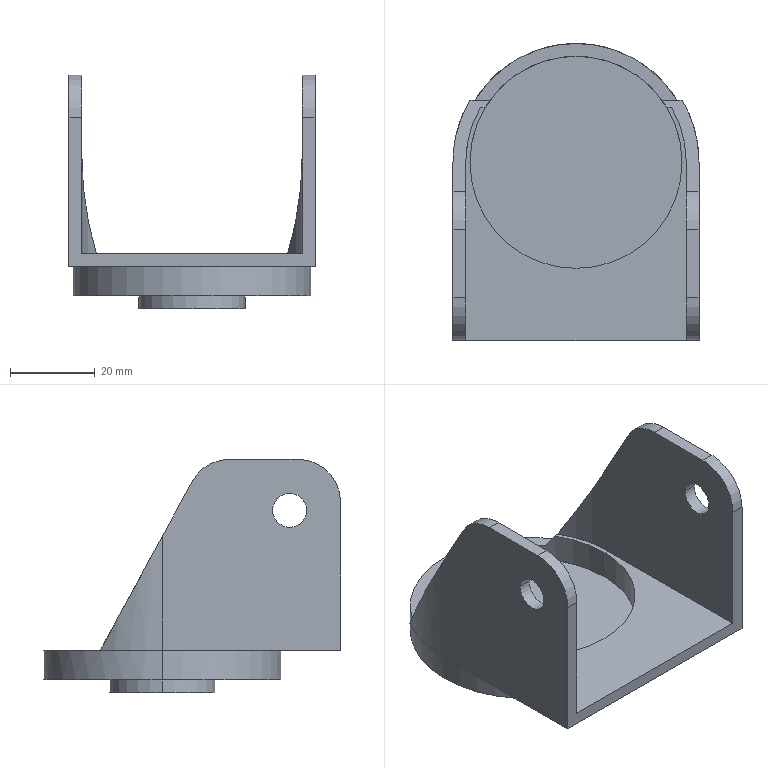Part | SolidWorks | features ICE 7, Extrusion 1, Fillet 1 | 1 solid | 33 faces | box 58 x 70 x 55 mm | volume 26099 mm3 | cylinder 18 | plane 15 | commonest cylinder face diameters 8 x4 20 x4 25 x2 50 x2 52 x2 56 x2
STEP:
#1=CARTESIAN_POINT('',(26.,-26.,43.));
#2=VERTEX_POINT('',#1);
#3=CARTESIAN_POINT('',(26.,-34.,43.));
#4=VERTEX_POINT('',#3);
#5=CARTESIAN_POINT('',(26.,-30.,43.));
#6=DIRECTION('',(-1.,0.,0.));
#7=DIRECTION('',(0.,-1.,0.));
#8=AXIS2_PLACEMENT_3D('',#5,#6,#7);
#9=CIRCLE('',#8,4.);
#10=EDGE_CURVE('',#2,#4,#9,.T.);
#11=ORIENTED_EDGE('',*,*,#10,.T.);
#12=CARTESIAN_POINT('',(29.,-34.,43.));
#13=VERTEX_POINT('',#12);
#14=CARTESIAN_POINT('',(-29.,-34.,43.));
#15=DIRECTION('',(1.,0.,0.));
#16=VECTOR('',#15,1000.);
#17=LINE('',#14,#16);
#18=EDGE_CURVE('',#4,#13,#17,.T.);
#19=ORIENTED_EDGE('',*,*,#18,.T.);
#20=CARTESIAN_POINT('',(29.,-26.,43.));
#21=VERTEX_POINT('',#20);
#22=CARTESIAN_POINT('',(29.,-30.,43.));
#23=DIRECTION('',(1.,0.,0.));
#24=DIRECTION('',(0.,1.,0.));
#25=AXIS2_PLACEMENT_3D('',#22,#23,#24);
#26=CIRCLE('',#25,4.);
#27=EDGE_CURVE('',#13,#21,#26,.T.);
#28=ORIENTED_EDGE('',*,*,#27,.T.);
#29=CARTESIAN_POINT('',(-29.,-26.,43.));
#30=DIRECTION('',(1.,0.,0.));
#31=VECTOR('',#30,1000.);
#32=LINE('',#29,#31);
#33=EDGE_CURVE('',#2,#21,#32,.T.);
#34=ORIENTED_EDGE('',*,*,#33,.F.);
#35=EDGE_LOOP('',(#11,#19,#28,#34));
#36=FACE_OUTER_BOUND('',#35,.T.);
#37=CARTESIAN_POINT('',(-29.,-30.,43.));
#38=DIRECTION('',(1.,0.,0.));
#39=DIRECTION('',(0.,1.,0.));
#40=AXIS2_PLACEMENT_3D('',#37,#38,#39);
#41=CYLINDRICAL_SURFACE('',#40,4.);
#42=ADVANCED_FACE('',(#36),#41,.F.);
#43=CARTESIAN_POINT('',(-29.,-34.,43.));
#44=VERTEX_POINT('',#43);
#45=CARTESIAN_POINT('',(-29.,-26.,43.));
#46=VERTEX_POINT('',#45);
#47=CARTESIAN_POINT('',(-29.,-30.,43.));
#48=DIRECTION('',(1.,0.,0.));
#49=DIRECTION('',(0.,1.,0.));
#50=AXIS2_PLACEMENT_3D('',#47,#48,#49);
#51=CIRCLE('',#50,4.);
#52=EDGE_CURVE('',#44,#46,#51,.T.);
#53=ORIENTED_EDGE('',*,*,#52,.F.);
#54=CARTESIAN_POINT('',(-26.,-34.,43.));
#55=VERTEX_POINT('',#54);
#56=CARTESIAN_POINT('',(-29.,-34.,43.));
#57=DIRECTION('',(1.,0.,0.));
#58=VECTOR('',#57,1000.);
#59=LINE('',#56,#58);
#60=EDGE_CURVE('',#44,#55,#59,.T.);
#61=ORIENTED_EDGE('',*,*,#60,.T.);
#62=CARTESIAN_POINT('',(-26.,-26.,43.));
#63=VERTEX_POINT('',#62);
#64=CARTESIAN_POINT('',(-26.,-30.,43.));
#65=DIRECTION('',(1.,0.,0.));
#66=DIRECTION('',(0.,0.,-1.));
#67=AXIS2_PLACEMENT_3D('',#64,#65,#66);
#68=CIRCLE('',#67,4.);
#69=EDGE_CURVE('',#55,#63,#68,.T.);
#70=ORIENTED_EDGE('',*,*,#69,.T.);
#71=CARTESIAN_POINT('',(-29.,-26.,43.));
#72=DIRECTION('',(1.,0.,0.));
#73=VECTOR('',#72,1000.);
#74=LINE('',#71,#73);
#75=EDGE_CURVE('',#46,#63,#74,.T.);
#76=ORIENTED_EDGE('',*,*,#75,.F.);
#77=EDGE_LOOP('',(#53,#61,#70,#76));
#78=FACE_OUTER_BOUND('',#77,.T.);
#79=CARTESIAN_POINT('',(-29.,-30.,43.));
#80=DIRECTION('',(1.,0.,0.));
#81=DIRECTION('',(0.,1.,0.));
#82=AXIS2_PLACEMENT_3D('',#79,#80,#81);
#83=CYLINDRICAL_SURFACE('',#82,4.);
#84=ADVANCED_FACE('',(#78),#83,.F.);
#85=CARTESIAN_POINT('',(-25.,0.,6.));
#86=VERTEX_POINT('',#85);
#87=CARTESIAN_POINT('',(25.,0.,6.));
#88=VERTEX_POINT('',#87);
#89=CARTESIAN_POINT('',(0.,0.,6.));
#90=DIRECTION('',(0.,0.,1.));
#91=DIRECTION('',(1.,0.,0.));
#92=AXIS2_PLACEMENT_3D('',#89,#90,#91);
#93=CIRCLE('',#92,25.);
#94=EDGE_CURVE('',#86,#88,#93,.T.);
#95=ORIENTED_EDGE('',*,*,#94,.F.);
#96=CARTESIAN_POINT('',(-25.,0.,13.));
#97=VERTEX_POINT('',#96);
#98=CARTESIAN_POINT('',(-25.,0.,6.));
#99=DIRECTION('',(0.,0.,1.));
#100=VECTOR('',#99,1000.);
#101=LINE('',#98,#100);
#102=EDGE_CURVE('',#86,#97,#101,.T.);
#103=ORIENTED_EDGE('',*,*,#102,.T.);
#104=CARTESIAN_POINT('',(25.,0.,13.));
#105=VERTEX_POINT('',#104);
#106=CARTESIAN_POINT('',(0.,0.,13.));
#107=DIRECTION('',(0.,0.,1.));
#108=DIRECTION('',(1.,0.,0.));
#109=AXIS2_PLACEMENT_3D('',#106,#107,#108);
#110=CIRCLE('',#109,25.);
#111=EDGE_CURVE('',#97,#105,#110,.T.);
#112=ORIENTED_EDGE('',*,*,#111,.T.);
#113=CARTESIAN_POINT('',(25.,0.,6.));
#114=DIRECTION('',(0.,0.,1.));
#115=VECTOR('',#114,1000.);
#116=LINE('',#113,#115);
#117=EDGE_CURVE('',#88,#105,#116,.T.);
#118=ORIENTED_EDGE('',*,*,#117,.F.);
#119=EDGE_LOOP('',(#95,#103,#112,#118));
#120=FACE_OUTER_BOUND('',#119,.T.);
#121=CARTESIAN_POINT('',(0.,0.,6.));
#122=DIRECTION('',(0.,0.,1.));
#123=DIRECTION('',(1.,0.,0.));
#124=AXIS2_PLACEMENT_3D('',#121,#122,#123);
#125=CYLINDRICAL_SURFACE('',#124,25.);
#126=ADVANCED_FACE('',(#120),#125,.F.);
#127=CARTESIAN_POINT('',(12.5,0.,3.));
#128=VERTEX_POINT('',#127);
#129=CARTESIAN_POINT('',(-12.5,0.,3.));
#130=VERTEX_POINT('',#129);
#131=CARTESIAN_POINT('',(0.,0.,3.));
#132=DIRECTION('',(0.,0.,1.));
#133=DIRECTION('',(1.,0.,0.));
#134=AXIS2_PLACEMENT_3D('',#131,#132,#133);
#135=CIRCLE('',#134,12.5);
#136=EDGE_CURVE('',#128,#130,#135,.T.);
#137=ORIENTED_EDGE('',*,*,#136,.F.);
#138=CARTESIAN_POINT('',(12.5,0.,0.));
#139=VERTEX_POINT('',#138);
#140=CARTESIAN_POINT('',(12.5,0.,3.));
#141=DIRECTION('',(0.,0.,-1.));
#142=VECTOR('',#141,1000.);
#143=LINE('',#140,#142);
#144=EDGE_CURVE('',#128,#139,#143,.T.);
#145=ORIENTED_EDGE('',*,*,#144,.T.);
#146=CARTESIAN_POINT('',(-12.5,0.,0.));
#147=VERTEX_POINT('',#146);
#148=CARTESIAN_POINT('',(0.,0.,0.));
#149=DIRECTION('',(0.,0.,1.));
#150=DIRECTION('',(1.,0.,0.));
#151=AXIS2_PLACEMENT_3D('',#148,#149,#150);
#152=CIRCLE('',#151,12.5);
#153=EDGE_CURVE('',#139,#147,#152,.T.);
#154=ORIENTED_EDGE('',*,*,#153,.T.);
#155=CARTESIAN_POINT('',(-12.5,0.,3.));
#156=DIRECTION('',(0.,0.,-1.));
#157=VECTOR('',#156,1000.);
#158=LINE('',#155,#157);
#159=EDGE_CURVE('',#130,#147,#158,.T.);
#160=ORIENTED_EDGE('',*,*,#159,.F.);
#161=EDGE_LOOP('',(#137,#145,#154,#160));
#162=FACE_OUTER_BOUND('',#161,.T.);
#163=CARTESIAN_POINT('',(0.,0.,3.));
#164=DIRECTION('',(0.,0.,-1.));
#165=DIRECTION('',(-1.,0.,0.));
#166=AXIS2_PLACEMENT_3D('',#163,#164,#165);
#167=CYLINDRICAL_SURFACE('',#166,12.5);
#168=ADVANCED_FACE('',(#162),#167,.T.);
#169=CARTESIAN_POINT('',(28.,0.,10.));
#170=VERTEX_POINT('',#169);
#171=CARTESIAN_POINT('',(23.886,14.61,10.));
#172=VERTEX_POINT('',#171);
#173=CARTESIAN_POINT('',(0.,0.,10.));
#174=DIRECTION('',(0.,0.,1.));
#175=DIRECTION('',(1.,0.,0.));
#176=AXIS2_PLACEMENT_3D('',#173,#174,#175);
#177=CIRCLE('',#176,28.);
#178=EDGE_CURVE('',#170,#172,#177,.T.);
#179=ORIENTED_EDGE('',*,*,#178,.F.);
#180=CARTESIAN_POINT('',(28.,0.,3.));
#181=VERTEX_POINT('',#180);
#182=CARTESIAN_POINT('',(28.,0.,13.));
#183=DIRECTION('',(0.,0.,-1.));
#184=VECTOR('',#183,1000.);
#185=LINE('',#182,#184);
#186=EDGE_CURVE('',#170,#181,#185,.T.);
#187=ORIENTED_EDGE('',*,*,#186,.T.);
#188=CARTESIAN_POINT('',(-28.,0.,3.));
#189=VERTEX_POINT('',#188);
#190=CARTESIAN_POINT('',(0.,0.,3.));
#191=DIRECTION('',(0.,0.,1.));
#192=DIRECTION('',(1.,0.,0.));
#193=AXIS2_PLACEMENT_3D('',#190,#191,#192);
#194=CIRCLE('',#193,28.);
#195=EDGE_CURVE('',#181,#189,#194,.T.);
#196=ORIENTED_EDGE('',*,*,#195,.T.);
#197=CARTESIAN_POINT('',(-28.,0.,10.));
#198=VERTEX_POINT('',#197);
#199=CARTESIAN_POINT('',(-28.,0.,13.));
#200=DIRECTION('',(0.,0.,-1.));
#201=VECTOR('',#200,1000.);
#202=LINE('',#199,#201);
#203=EDGE_CURVE('',#198,#189,#202,.T.);
#204=ORIENTED_EDGE('',*,*,#203,.F.);
#205=CARTESIAN_POINT('',(-23.886,14.61,10.));
#206=VERTEX_POINT('',#205);
#207=CARTESIAN_POINT('',(0.,0.,10.));
#208=DIRECTION('',(0.,0.,1.));
#209=DIRECTION('',(1.,0.,0.));
#210=AXIS2_PLACEMENT_3D('',#207,#208,#209);
#211=CIRCLE('',#210,28.);
#212=EDGE_CURVE('',#206,#198,#211,.T.);
#213=ORIENTED_EDGE('',*,*,#212,.F.);
#214=CARTESIAN_POINT('',(0.,0.,10.));
#215=DIRECTION('',(0.,0.,1.));
#216=DIRECTION('',(1.,0.,0.));
#217=AXIS2_PLACEMENT_3D('',#214,#215,#216);
#218=CIRCLE('',#217,28.);
#219=EDGE_CURVE('',#172,#206,#218,.T.);
#220=ORIENTED_EDGE('',*,*,#219,.F.);
#221=EDGE_LOOP('',(#179,#187,#196,#204,#213,#220));
#222=FACE_OUTER_BOUND('',#221,.T.);
#223=CARTESIAN_POINT('',(0.,0.,13.));
#224=DIRECTION('',(0.,0.,-1.));
#225=DIRECTION('',(-1.,0.,0.));
#226=AXIS2_PLACEMENT_3D('',#223,#224,#225);
#227=CYLINDRICAL_SURFACE('',#226,28.);
#228=ADVANCED_FACE('',(#222),#227,.T.);
#229=CARTESIAN_POINT('',(29.,0.,36.854));
#230=VERTEX_POINT('',#229);
#231=CARTESIAN_POINT('',(25.051,14.61,10.));
#232=VERTEX_POINT('',#231);
#233=CARTESIAN_POINT('',(29.,0.,36.854));
#234=CARTESIAN_POINT('',(29.,5.164,27.362));
#235=CARTESIAN_POINT('',(27.653,10.149,18.199));
#236=CARTESIAN_POINT('',(25.051,14.61,10.));
#237=(BOUNDED_CURVE()B_SPLINE_CURVE(3,(#233,#234,#235,#236),.UNSPECIFIED.,.F.,.F.)B_SPLINE_CURVE_WITH_KNOTS((4,4),(1.571,2.099),.UNSPECIFIED.)CURVE()GEOMETRIC_REPRESENTATION_ITEM()RATIONAL_B_SPLINE_CURVE((1.,0.9769,0.9769,1.))REPRESENTATION_ITEM(''));
#238=EDGE_CURVE('',#230,#232,#237,.T.);
#239=ORIENTED_EDGE('',*,*,#238,.F.);
#240=CARTESIAN_POINT('',(29.,0.,10.));
#241=VERTEX_POINT('',#240);
#242=CARTESIAN_POINT('',(29.,0.,10.));
#243=DIRECTION('',(0.,0.,1.));
#244=VECTOR('',#243,1000.);
#245=LINE('',#242,#244);
#246=EDGE_CURVE('',#241,#230,#245,.T.);
#247=ORIENTED_EDGE('',*,*,#246,.F.);
#248=CARTESIAN_POINT('',(0.,0.,10.));
#249=DIRECTION('',(0.,0.,1.));
#250=DIRECTION('',(1.,0.,0.));
#251=AXIS2_PLACEMENT_3D('',#248,#249,#250);
#252=CIRCLE('',#251,29.);
#253=EDGE_CURVE('',#241,#232,#252,.T.);
#254=ORIENTED_EDGE('',*,*,#253,.T.);
#255=EDGE_LOOP('',(#239,#247,#254));
#256=FACE_OUTER_BOUND('',#255,.T.);
#257=CARTESIAN_POINT('',(0.,0.,10.));
#258=DIRECTION('',(0.,0.,1.));
#259=DIRECTION('',(1.,0.,0.));
#260=AXIS2_PLACEMENT_3D('',#257,#258,#259);
#261=CYLINDRICAL_SURFACE('',#260,29.);
#262=ADVANCED_FACE('',(#256),#261,.T.);
#263=CARTESIAN_POINT('',(22.53,12.978,13.));
#264=VERTEX_POINT('',#263);
#265=CARTESIAN_POINT('',(26.,0.,36.854));
#266=VERTEX_POINT('',#265);
#267=CARTESIAN_POINT('',(22.53,12.978,13.));
#268=CARTESIAN_POINT('',(24.816,9.008,20.297));
#269=CARTESIAN_POINT('',(26.,4.582,28.432));
#270=CARTESIAN_POINT('',(26.,0.,36.854));
#271=(BOUNDED_CURVE()B_SPLINE_CURVE(3,(#267,#268,#269,#270),.UNSPECIFIED.,.F.,.F.)B_SPLINE_CURVE_WITH_KNOTS((4,4),(1.048,1.571),.UNSPECIFIED.)CURVE()GEOMETRIC_REPRESENTATION_ITEM()RATIONAL_B_SPLINE_CURVE((1.,0.9774,0.9774,1.))REPRESENTATION_ITEM(''));
#272=EDGE_CURVE('',#264,#266,#271,.T.);
#273=ORIENTED_EDGE('',*,*,#272,.F.);
#274=CARTESIAN_POINT('',(26.,0.,13.));
#275=VERTEX_POINT('',#274);
#276=CARTESIAN_POINT('',(0.,0.,13.));
#277=DIRECTION('',(0.,0.,1.));
#278=DIRECTION('',(1.,0.,0.));
#279=AXIS2_PLACEMENT_3D('',#276,#277,#278);
#280=CIRCLE('',#279,26.);
#281=EDGE_CURVE('',#275,#264,#280,.T.);
#282=ORIENTED_EDGE('',*,*,#281,.F.);
#283=CARTESIAN_POINT('',(26.,0.,55.));
#284=DIRECTION('',(0.,0.,-1.));
#285=VECTOR('',#284,1000.);
#286=LINE('',#283,#285);
#287=EDGE_CURVE('',#266,#275,#286,.T.);
#288=ORIENTED_EDGE('',*,*,#287,.F.);
#289=EDGE_LOOP('',(#273,#282,#288));
#290=FACE_OUTER_BOUND('',#289,.T.);
#291=CARTESIAN_POINT('',(0.,0.,55.));
#292=DIRECTION('',(0.,0.,-1.));
#293=DIRECTION('',(-1.,0.,0.));
#294=AXIS2_PLACEMENT_3D('',#291,#292,#293);
#295=CYLINDRICAL_SURFACE('',#294,26.);
#296=ADVANCED_FACE('',(#290),#295,.F.);
#297=CARTESIAN_POINT('',(-29.,-15.816,55.));
#298=VERTEX_POINT('',#297);
#299=CARTESIAN_POINT('',(-29.,-32.,55.));
#300=VERTEX_POINT('',#299);
#301=CARTESIAN_POINT('',(-29.,0.,55.));
#302=DIRECTION('',(0.,-1.,0.));
#303=VECTOR('',#302,1000.);
#304=LINE('',#301,#303);
#305=EDGE_CURVE('',#298,#300,#304,.T.);
#306=ORIENTED_EDGE('',*,*,#305,.T.);
#307=CARTESIAN_POINT('',(-26.,-32.,55.));
#308=VERTEX_POINT('',#307);
#309=CARTESIAN_POINT('',(0.,-32.,55.));
#310=DIRECTION('',(1.,0.,0.));
#311=VECTOR('',#310,1000.);
#312=LINE('',#309,#311);
#313=EDGE_CURVE('',#300,#308,#312,.T.);
#314=ORIENTED_EDGE('',*,*,#313,.T.);
#315=CARTESIAN_POINT('',(-26.,-15.816,55.));
#316=VERTEX_POINT('',#315);
#317=CARTESIAN_POINT('',(-26.,0.,55.));
#318=DIRECTION('',(0.,-1.,0.));
#319=VECTOR('',#318,1000.);
#320=LINE('',#317,#319);
#321=EDGE_CURVE('',#316,#308,#320,.T.);
#322=ORIENTED_EDGE('',*,*,#321,.F.);
#323=CARTESIAN_POINT('',(-29.,-15.816,55.));
#324=DIRECTION('',(-1.,0.,0.));
#325=VECTOR('',#324,1000.);
#326=LINE('',#323,#325);
#327=EDGE_CURVE('',#316,#298,#326,.T.);
#328=ORIENTED_EDGE('',*,*,#327,.T.);
#329=EDGE_LOOP('',(#306,#314,#322,#328));
#330=FACE_OUTER_BOUND('',#329,.T.);
#331=CARTESIAN_POINT('',(0.,0.,55.));
#332=DIRECTION('',(0.,0.,1.));
#333=DIRECTION('',(1.,0.,0.));
#334=AXIS2_PLACEMENT_3D('',#331,#332,#333);
#335=PLANE('',#334);
#336=ADVANCED_FACE('',(#330),#335,.T.);
#337=CARTESIAN_POINT('',(-22.53,12.978,13.));
#338=VERTEX_POINT('',#337);
#339=CARTESIAN_POINT('',(-21.368,12.978,13.));
#340=VERTEX_POINT('',#339);
#341=CARTESIAN_POINT('',(0.,12.978,13.));
#342=DIRECTION('',(1.,0.,0.));
#343=VECTOR('',#342,1000.);
#344=LINE('',#341,#343);
#345=EDGE_CURVE('',#338,#340,#344,.T.);
#346=ORIENTED_EDGE('',*,*,#345,.F.);
#347=CARTESIAN_POINT('',(-26.,0.,13.));
#348=VERTEX_POINT('',#347);
#349=CARTESIAN_POINT('',(0.,0.,13.));
#350=DIRECTION('',(0.,0.,1.));
#351=DIRECTION('',(1.,0.,0.));
#352=AXIS2_PLACEMENT_3D('',#349,#350,#351);
#353=CIRCLE('',#352,26.);
#354=EDGE_CURVE('',#338,#348,#353,.T.);
#355=ORIENTED_EDGE('',*,*,#354,.T.);
#356=CARTESIAN_POINT('',(-26.,-42.,13.));
#357=VERTEX_POINT('',#356);
#358=CARTESIAN_POINT('',(-26.,0.,13.));
#359=DIRECTION('',(0.,-1.,0.));
#360=VECTOR('',#359,1000.);
#361=LINE('',#358,#360);
#362=EDGE_CURVE('',#348,#357,#361,.T.);
#363=ORIENTED_EDGE('',*,*,#362,.T.);
#364=CARTESIAN_POINT('',(26.,-42.,13.));
#365=VERTEX_POINT('',#364);
#366=CARTESIAN_POINT('',(0.,-42.,13.));
#367=DIRECTION('',(1.,0.,0.));
#368=VECTOR('',#367,1000.);
#369=LINE('',#366,#368);
#370=EDGE_CURVE('',#357,#365,#369,.T.);
#371=ORIENTED_EDGE('',*,*,#370,.T.);
#372=CARTESIAN_POINT('',(26.,0.,13.));
#373=DIRECTION('',(0.,1.,0.));
#374=VECTOR('',#373,1000.);
#375=LINE('',#372,#374);
#376=EDGE_CURVE('',#365,#275,#375,.T.);
#377=ORIENTED_EDGE('',*,*,#376,.T.);
#378=ORIENTED_EDGE('',*,*,#281,.T.);
#379=CARTESIAN_POINT('',(21.368,12.978,13.));
#380=VERTEX_POINT('',#379);
#381=CARTESIAN_POINT('',(0.,12.978,13.));
#382=DIRECTION('',(1.,0.,0.));
#383=VECTOR('',#382,1000.);
#384=LINE('',#381,#383);
#385=EDGE_CURVE('',#380,#264,#384,.T.);
#386=ORIENTED_EDGE('',*,*,#385,.F.);
#387=CARTESIAN_POINT('',(0.,0.,13.));
#388=DIRECTION('',(0.,0.,1.));
#389=DIRECTION('',(1.,0.,0.));
#390=AXIS2_PLACEMENT_3D('',#387,#388,#389);
#391=CIRCLE('',#390,25.);
#392=EDGE_CURVE('',#105,#380,#391,.T.);
#393=ORIENTED_EDGE('',*,*,#392,.F.);
#394=ORIENTED_EDGE('',*,*,#111,.F.);
#395=CARTESIAN_POINT('',(0.,0.,13.));
#396=DIRECTION('',(0.,0.,1.));
#397=DIRECTION('',(1.,0.,0.));
#398=AXIS2_PLACEMENT_3D('',#395,#396,#397);
#399=CIRCLE('',#398,25.);
#400=EDGE_CURVE('',#340,#97,#399,.T.);
#401=ORIENTED_EDGE('',*,*,#400,.F.);
#402=EDGE_LOOP('',(#346,#355,#363,#371,#377,#378,#386,#393,#394,#401));
#403=FACE_OUTER_BOUND('',#402,.T.);
#404=CARTESIAN_POINT('',(0.,0.,13.));
#405=DIRECTION('',(0.,0.,1.));
#406=DIRECTION('',(1.,0.,0.));
#407=AXIS2_PLACEMENT_3D('',#404,#405,#406);
#408=PLANE('',#407);
#409=ADVANCED_FACE('',(#403),#408,.T.);
#410=CARTESIAN_POINT('',(-25.051,14.61,10.));
#411=VERTEX_POINT('',#410);
#412=CARTESIAN_POINT('',(-29.,0.,36.854));
#413=VERTEX_POINT('',#412);
#414=CARTESIAN_POINT('',(-25.051,14.61,10.));
#415=CARTESIAN_POINT('',(-27.653,10.149,18.199));
#416=CARTESIAN_POINT('',(-29.,5.164,27.362));
#417=CARTESIAN_POINT('',(-29.,0.,36.854));
#418=(BOUNDED_CURVE()B_SPLINE_CURVE(3,(#414,#415,#416,#417),.UNSPECIFIED.,.F.,.F.)B_SPLINE_CURVE_WITH_KNOTS((4,4),(4.184,4.712),.UNSPECIFIED.)CURVE()GEOMETRIC_REPRESENTATION_ITEM()RATIONAL_B_SPLINE_CURVE((1.,0.9769,0.9769,1.))REPRESENTATION_ITEM(''));
#419=EDGE_CURVE('',#411,#413,#418,.T.);
#420=ORIENTED_EDGE('',*,*,#419,.F.);
#421=CARTESIAN_POINT('',(-29.,0.,10.));
#422=VERTEX_POINT('',#421);
#423=CARTESIAN_POINT('',(0.,0.,10.));
#424=DIRECTION('',(0.,0.,1.));
#425=DIRECTION('',(1.,0.,0.));
#426=AXIS2_PLACEMENT_3D('',#423,#424,#425);
#427=CIRCLE('',#426,29.);
#428=EDGE_CURVE('',#411,#422,#427,.T.);
#429=ORIENTED_EDGE('',*,*,#428,.T.);
#430=CARTESIAN_POINT('',(-29.,0.,10.));
#431=DIRECTION('',(0.,0.,1.));
#432=VECTOR('',#431,1000.);
#433=LINE('',#430,#432);
#434=EDGE_CURVE('',#422,#413,#433,.T.);
#435=ORIENTED_EDGE('',*,*,#434,.T.);
#436=EDGE_LOOP('',(#420,#429,#435));
#437=FACE_OUTER_BOUND('',#436,.T.);
#438=CARTESIAN_POINT('',(0.,0.,10.));
#439=DIRECTION('',(0.,0.,1.));
#440=DIRECTION('',(1.,0.,0.));
#441=AXIS2_PLACEMENT_3D('',#438,#439,#440);
#442=CYLINDRICAL_SURFACE('',#441,29.);
#443=ADVANCED_FACE('',(#437),#442,.T.);
#444=ORIENTED_EDGE('',*,*,#186,.F.);
#445=CARTESIAN_POINT('',(0.,0.,10.));
#446=DIRECTION('',(0.,0.,1.));
#447=DIRECTION('',(1.,0.,0.));
#448=AXIS2_PLACEMENT_3D('',#445,#446,#447);
#449=CIRCLE('',#448,28.);
#450=EDGE_CURVE('',#198,#170,#449,.T.);
#451=ORIENTED_EDGE('',*,*,#450,.F.);
#452=ORIENTED_EDGE('',*,*,#203,.T.);
#453=CARTESIAN_POINT('',(0.,0.,3.));
#454=DIRECTION('',(0.,0.,1.));
#455=DIRECTION('',(1.,0.,0.));
#456=AXIS2_PLACEMENT_3D('',#453,#454,#455);
#457=CIRCLE('',#456,28.);
#458=EDGE_CURVE('',#189,#181,#457,.T.);
#459=ORIENTED_EDGE('',*,*,#458,.T.);
#460=EDGE_LOOP('',(#444,#451,#452,#459));
#461=FACE_OUTER_BOUND('',#460,.T.);
#462=CARTESIAN_POINT('',(0.,0.,13.));
#463=DIRECTION('',(0.,0.,-1.));
#464=DIRECTION('',(-1.,0.,0.));
#465=AXIS2_PLACEMENT_3D('',#462,#463,#464);
#466=CYLINDRICAL_SURFACE('',#465,28.);
#467=ADVANCED_FACE('',(#461),#466,.T.);
#468=ORIENTED_EDGE('',*,*,#144,.F.);
#469=CARTESIAN_POINT('',(0.,0.,3.));
#470=DIRECTION('',(0.,0.,1.));
#471=DIRECTION('',(1.,0.,0.));
#472=AXIS2_PLACEMENT_3D('',#469,#470,#471);
#473=CIRCLE('',#472,12.5);
#474=EDGE_CURVE('',#130,#128,#473,.T.);
#475=ORIENTED_EDGE('',*,*,#474,.F.);
#476=ORIENTED_EDGE('',*,*,#159,.T.);
#477=CARTESIAN_POINT('',(0.,0.,0.));
#478=DIRECTION('',(0.,0.,1.));
#479=DIRECTION('',(1.,0.,0.));
#480=AXIS2_PLACEMENT_3D('',#477,#478,#479);
#481=CIRCLE('',#480,12.5);
#482=EDGE_CURVE('',#147,#139,#481,.T.);
#483=ORIENTED_EDGE('',*,*,#482,.T.);
#484=EDGE_LOOP('',(#468,#475,#476,#483));
#485=FACE_OUTER_BOUND('',#484,.T.);
#486=CARTESIAN_POINT('',(0.,0.,3.));
#487=DIRECTION('',(0.,0.,-1.));
#488=DIRECTION('',(-1.,0.,0.));
#489=AXIS2_PLACEMENT_3D('',#486,#487,#488);
#490=CYLINDRICAL_SURFACE('',#489,12.5);
#491=ADVANCED_FACE('',(#485),#490,.T.);
#492=ORIENTED_EDGE('',*,*,#482,.F.);
#493=ORIENTED_EDGE('',*,*,#153,.F.);
#494=EDGE_LOOP('',(#492,#493));
#495=FACE_OUTER_BOUND('',#494,.T.);
#496=CARTESIAN_POINT('',(0.,0.,0.));
#497=DIRECTION('',(0.,0.,1.));
#498=DIRECTION('',(1.,0.,0.));
#499=AXIS2_PLACEMENT_3D('',#496,#497,#498);
#500=PLANE('',#499);
#501=ADVANCED_FACE('',(#495),#500,.F.);
#502=ORIENTED_EDGE('',*,*,#458,.F.);
#503=ORIENTED_EDGE('',*,*,#195,.F.);
#504=EDGE_LOOP('',(#502,#503));
#505=FACE_OUTER_BOUND('',#504,.T.);
#506=ORIENTED_EDGE('',*,*,#474,.T.);
#507=ORIENTED_EDGE('',*,*,#136,.T.);
#508=EDGE_LOOP('',(#506,#507));
#509=FACE_BOUND('',#508,.T.);
#510=CARTESIAN_POINT('',(0.,0.,3.));
#511=DIRECTION('',(0.,0.,1.));
#512=DIRECTION('',(1.,0.,0.));
#513=AXIS2_PLACEMENT_3D('',#510,#511,#512);
#514=PLANE('',#513);
#515=ADVANCED_FACE('',(#505,#509),#514,.F.);
#516=ORIENTED_EDGE('',*,*,#428,.F.);
#517=CARTESIAN_POINT('',(-29.,14.61,10.));
#518=DIRECTION('',(1.,0.,0.));
#519=VECTOR('',#518,1000.);
#520=LINE('',#517,#519);
#521=EDGE_CURVE('',#411,#206,#520,.T.);
#522=ORIENTED_EDGE('',*,*,#521,.T.);
#523=ORIENTED_EDGE('',*,*,#212,.T.);
#524=ORIENTED_EDGE('',*,*,#450,.T.);
#525=ORIENTED_EDGE('',*,*,#178,.T.);
#526=CARTESIAN_POINT('',(-29.,14.61,10.));
#527=DIRECTION('',(1.,0.,0.));
#528=VECTOR('',#527,1000.);
#529=LINE('',#526,#528);
#530=EDGE_CURVE('',#172,#232,#529,.T.);
#531=ORIENTED_EDGE('',*,*,#530,.T.);
#532=ORIENTED_EDGE('',*,*,#253,.F.);
#533=CARTESIAN_POINT('',(29.,-42.,10.));
#534=VERTEX_POINT('',#533);
#535=CARTESIAN_POINT('',(29.,0.,10.));
#536=DIRECTION('',(0.,-1.,0.));
#537=VECTOR('',#536,1000.);
#538=LINE('',#535,#537);
#539=EDGE_CURVE('',#241,#534,#538,.T.);
#540=ORIENTED_EDGE('',*,*,#539,.T.);
#541=CARTESIAN_POINT('',(-29.,-42.,10.));
#542=VERTEX_POINT('',#541);
#543=CARTESIAN_POINT('',(0.,-42.,10.));
#544=DIRECTION('',(1.,0.,0.));
#545=VECTOR('',#544,1000.);
#546=LINE('',#543,#545);
#547=EDGE_CURVE('',#542,#534,#546,.T.);
#548=ORIENTED_EDGE('',*,*,#547,.F.);
#549=CARTESIAN_POINT('',(-29.,0.,10.));
#550=DIRECTION('',(0.,-1.,0.));
#551=VECTOR('',#550,1000.);
#552=LINE('',#549,#551);
#553=EDGE_CURVE('',#422,#542,#552,.T.);
#554=ORIENTED_EDGE('',*,*,#553,.F.);
#555=EDGE_LOOP('',(#516,#522,#523,#524,#525,#531,#532,#540,#548,#554));
#556=FACE_OUTER_BOUND('',#555,.T.);
#557=CARTESIAN_POINT('',(0.,0.,10.));
#558=DIRECTION('',(0.,0.,1.));
#559=DIRECTION('',(1.,0.,0.));
#560=AXIS2_PLACEMENT_3D('',#557,#558,#559);
#561=PLANE('',#560);
#562=ADVANCED_FACE('',(#556),#561,.F.);
#563=CARTESIAN_POINT('',(0.,0.,6.));
#564=DIRECTION('',(0.,0.,1.));
#565=DIRECTION('',(1.,0.,0.));
#566=AXIS2_PLACEMENT_3D('',#563,#564,#565);
#567=CIRCLE('',#566,25.);
#568=EDGE_CURVE('',#88,#86,#567,.T.);
#569=ORIENTED_EDGE('',*,*,#568,.T.);
#570=ORIENTED_EDGE('',*,*,#94,.T.);
#571=EDGE_LOOP('',(#569,#570));
#572=FACE_OUTER_BOUND('',#571,.T.);
#573=CARTESIAN_POINT('',(0.,0.,6.));
#574=DIRECTION('',(0.,0.,1.));
#575=DIRECTION('',(1.,0.,0.));
#576=AXIS2_PLACEMENT_3D('',#573,#574,#575);
#577=PLANE('',#576);
#578=ADVANCED_FACE('',(#572),#577,.T.);
#579=ORIENTED_EDGE('',*,*,#102,.F.);
#580=ORIENTED_EDGE('',*,*,#568,.F.);
#581=ORIENTED_EDGE('',*,*,#117,.T.);
#582=ORIENTED_EDGE('',*,*,#392,.T.);
#583=CARTESIAN_POINT('',(20.287,14.61,10.));
#584=VERTEX_POINT('',#583);
#585=CARTESIAN_POINT('',(21.368,12.978,13.));
#586=CARTESIAN_POINT('',(21.029,13.536,11.974));
#587=CARTESIAN_POINT('',(20.668,14.08,10.974));
#588=CARTESIAN_POINT('',(20.287,14.61,10.));
#589=(BOUNDED_CURVE()B_SPLINE_CURVE(3,(#585,#586,#587,#588),.UNSPECIFIED.,.F.,.T.)B_SPLINE_CURVE_WITH_KNOTS((4,4),(2.117,2.195),.UNSPECIFIED.)CURVE()GEOMETRIC_REPRESENTATION_ITEM()RATIONAL_B_SPLINE_CURVE((1.,0.9995,0.9995,1.))REPRESENTATION_ITEM(''));
#590=EDGE_CURVE('',#380,#584,#589,.T.);
#591=ORIENTED_EDGE('',*,*,#590,.T.);
#592=CARTESIAN_POINT('',(-20.287,14.61,10.));
#593=VERTEX_POINT('',#592);
#594=CARTESIAN_POINT('',(0.,0.,10.));
#595=DIRECTION('',(0.,0.,1.));
#596=DIRECTION('',(-1.,0.,0.));
#597=AXIS2_PLACEMENT_3D('',#594,#595,#596);
#598=CIRCLE('',#597,25.);
#599=EDGE_CURVE('',#584,#593,#598,.T.);
#600=ORIENTED_EDGE('',*,*,#599,.T.);
#601=CARTESIAN_POINT('',(-20.287,14.61,10.));
#602=CARTESIAN_POINT('',(-20.668,14.08,10.974));
#603=CARTESIAN_POINT('',(-21.029,13.536,11.974));
#604=CARTESIAN_POINT('',(-21.368,12.978,13.));
#605=(BOUNDED_CURVE()B_SPLINE_CURVE(3,(#601,#602,#603,#604),.UNSPECIFIED.,.F.,.F.)B_SPLINE_CURVE_WITH_KNOTS((4,4),(4.088,4.167),.UNSPECIFIED.)CURVE()GEOMETRIC_REPRESENTATION_ITEM()RATIONAL_B_SPLINE_CURVE((1.,0.9995,0.9995,1.))REPRESENTATION_ITEM(''));
#606=EDGE_CURVE('',#593,#340,#605,.T.);
#607=ORIENTED_EDGE('',*,*,#606,.T.);
#608=ORIENTED_EDGE('',*,*,#400,.T.);
#609=EDGE_LOOP('',(#579,#580,#581,#582,#591,#600,#607,#608));
#610=FACE_OUTER_BOUND('',#609,.T.);
#611=CARTESIAN_POINT('',(0.,0.,6.));
#612=DIRECTION('',(0.,0.,1.));
#613=DIRECTION('',(1.,0.,0.));
#614=AXIS2_PLACEMENT_3D('',#611,#612,#613);
#615=CYLINDRICAL_SURFACE('',#614,25.);
#616=ADVANCED_FACE('',(#610),#615,.F.);
#617=CARTESIAN_POINT('',(29.,-30.,43.));
#618=DIRECTION('',(1.,0.,0.));
#619=DIRECTION('',(0.,1.,0.));
#620=AXIS2_PLACEMENT_3D('',#617,#618,#619);
#621=CIRCLE('',#620,4.);
#622=EDGE_CURVE('',#21,#13,#621,.T.);
#623=ORIENTED_EDGE('',*,*,#622,.F.);
#624=ORIENTED_EDGE('',*,*,#27,.F.);
#625=EDGE_LOOP('',(#623,#624));
#626=FACE_BOUND('',#625,.T.);
#627=CARTESIAN_POINT('',(29.,-32.,55.));
#628=VERTEX_POINT('',#627);
#629=CARTESIAN_POINT('',(29.,-15.816,55.));
#630=VERTEX_POINT('',#629);
#631=CARTESIAN_POINT('',(29.,0.,55.));
#632=DIRECTION('',(0.,1.,0.));
#633=VECTOR('',#632,1000.);
#634=LINE('',#631,#633);
#635=EDGE_CURVE('',#628,#630,#634,.T.);
#636=ORIENTED_EDGE('',*,*,#635,.F.);
#637=CARTESIAN_POINT('',(29.,-42.,45.));
#638=VERTEX_POINT('',#637);
#639=CARTESIAN_POINT('',(29.,-32.,45.));
#640=DIRECTION('',(1.,0.,0.));
#641=DIRECTION('',(0.,-1.,0.));
#642=AXIS2_PLACEMENT_3D('',#639,#640,#641);
#643=CIRCLE('',#642,10.);
#644=EDGE_CURVE('',#628,#638,#643,.T.);
#645=ORIENTED_EDGE('',*,*,#644,.T.);
#646=CARTESIAN_POINT('',(29.,-42.,10.));
#647=DIRECTION('',(0.,0.,1.));
#648=VECTOR('',#647,1000.);
#649=LINE('',#646,#648);
#650=EDGE_CURVE('',#534,#638,#649,.T.);
#651=ORIENTED_EDGE('',*,*,#650,.F.);
#652=ORIENTED_EDGE('',*,*,#539,.F.);
#653=ORIENTED_EDGE('',*,*,#246,.T.);
#654=CARTESIAN_POINT('',(29.,-7.032,49.779));
#655=VERTEX_POINT('',#654);
#656=CARTESIAN_POINT('',(29.,-9.873,55.));
#657=DIRECTION('',(0.,0.4779,-0.8784));
#658=VECTOR('',#657,1000.);
#659=LINE('',#656,#658);
#660=EDGE_CURVE('',#655,#230,#659,.T.);
#661=ORIENTED_EDGE('',*,*,#660,.F.);
#662=CARTESIAN_POINT('',(29.,-15.816,45.));
#663=DIRECTION('',(1.,0.,0.));
#664=DIRECTION('',(0.,-1.,0.));
#665=AXIS2_PLACEMENT_3D('',#662,#663,#664);
#666=CIRCLE('',#665,10.);
#667=EDGE_CURVE('',#655,#630,#666,.T.);
#668=ORIENTED_EDGE('',*,*,#667,.T.);
#669=EDGE_LOOP('',(#636,#645,#651,#652,#653,#661,#668));
#670=FACE_OUTER_BOUND('',#669,.T.);
#671=CARTESIAN_POINT('',(29.,0.,10.));
#672=DIRECTION('',(-1.,0.,0.));
#673=DIRECTION('',(0.,-1.,0.));
#674=AXIS2_PLACEMENT_3D('',#671,#672,#673);
#675=PLANE('',#674);
#676=ADVANCED_FACE('',(#626,#670),#675,.F.);
#677=ORIENTED_EDGE('',*,*,#650,.T.);
#678=CARTESIAN_POINT('',(26.,-42.,45.));
#679=VERTEX_POINT('',#678);
#680=CARTESIAN_POINT('',(0.,-42.,45.));
#681=DIRECTION('',(-1.,0.,0.));
#682=VECTOR('',#681,1000.);
#683=LINE('',#680,#682);
#684=EDGE_CURVE('',#638,#679,#683,.T.);
#685=ORIENTED_EDGE('',*,*,#684,.T.);
#686=CARTESIAN_POINT('',(26.,-42.,55.));
#687=DIRECTION('',(0.,0.,-1.));
#688=VECTOR('',#687,1000.);
#689=LINE('',#686,#688);
#690=EDGE_CURVE('',#679,#365,#689,.T.);
#691=ORIENTED_EDGE('',*,*,#690,.T.);
#692=ORIENTED_EDGE('',*,*,#370,.F.);
#693=CARTESIAN_POINT('',(-26.,-42.,45.));
#694=VERTEX_POINT('',#693);
#695=CARTESIAN_POINT('',(-26.,-42.,55.));
#696=DIRECTION('',(0.,0.,-1.));
#697=VECTOR('',#696,1000.);
#698=LINE('',#695,#697);
#699=EDGE_CURVE('',#694,#357,#698,.T.);
#700=ORIENTED_EDGE('',*,*,#699,.F.);
#701=CARTESIAN_POINT('',(-29.,-42.,45.));
#702=VERTEX_POINT('',#701);
#703=CARTESIAN_POINT('',(0.,-42.,45.));
#704=DIRECTION('',(-1.,0.,0.));
#705=VECTOR('',#704,1000.);
#706=LINE('',#703,#705);
#707=EDGE_CURVE('',#694,#702,#706,.T.);
#708=ORIENTED_EDGE('',*,*,#707,.T.);
#709=CARTESIAN_POINT('',(-29.,-42.,10.));
#710=DIRECTION('',(0.,0.,1.));
#711=VECTOR('',#710,1000.);
#712=LINE('',#709,#711);
#713=EDGE_CURVE('',#542,#702,#712,.T.);
#714=ORIENTED_EDGE('',*,*,#713,.F.);
#715=ORIENTED_EDGE('',*,*,#547,.T.);
#716=EDGE_LOOP('',(#677,#685,#691,#692,#700,#708,#714,#715));
#717=FACE_OUTER_BOUND('',#716,.T.);
#718=CARTESIAN_POINT('',(0.,-42.,10.));
#719=DIRECTION('',(0.,-1.,0.));
#720=DIRECTION('',(0.,0.,-1.));
#721=AXIS2_PLACEMENT_3D('',#718,#719,#720);
#722=PLANE('',#721);
#723=ADVANCED_FACE('',(#717),#722,.T.);
#724=CARTESIAN_POINT('',(-29.,-30.,43.));
#725=DIRECTION('',(1.,0.,0.));
#726=DIRECTION('',(0.,1.,0.));
#727=AXIS2_PLACEMENT_3D('',#724,#725,#726);
#728=CIRCLE('',#727,4.);
#729=EDGE_CURVE('',#46,#44,#728,.T.);
#730=ORIENTED_EDGE('',*,*,#729,.T.);
#731=ORIENTED_EDGE('',*,*,#52,.T.);
#732=EDGE_LOOP('',(#730,#731));
#733=FACE_BOUND('',#732,.T.);
#734=ORIENTED_EDGE('',*,*,#713,.T.);
#735=CARTESIAN_POINT('',(-29.,-32.,45.));
#736=DIRECTION('',(-1.,0.,0.));
#737=DIRECTION('',(0.,-1.,0.));
#738=AXIS2_PLACEMENT_3D('',#735,#736,#737);
#739=CIRCLE('',#738,10.);
#740=EDGE_CURVE('',#702,#300,#739,.T.);
#741=ORIENTED_EDGE('',*,*,#740,.T.);
#742=ORIENTED_EDGE('',*,*,#305,.F.);
#743=CARTESIAN_POINT('',(-29.,-7.032,49.779));
#744=VERTEX_POINT('',#743);
#745=CARTESIAN_POINT('',(-29.,-15.816,45.));
#746=DIRECTION('',(-1.,0.,0.));
#747=DIRECTION('',(0.,-1.,0.));
#748=AXIS2_PLACEMENT_3D('',#745,#746,#747);
#749=CIRCLE('',#748,10.);
#750=EDGE_CURVE('',#298,#744,#749,.T.);
#751=ORIENTED_EDGE('',*,*,#750,.T.);
#752=CARTESIAN_POINT('',(-29.,-9.873,55.));
#753=DIRECTION('',(0.,0.4779,-0.8784));
#754=VECTOR('',#753,1000.);
#755=LINE('',#752,#754);
#756=EDGE_CURVE('',#744,#413,#755,.T.);
#757=ORIENTED_EDGE('',*,*,#756,.T.);
#758=ORIENTED_EDGE('',*,*,#434,.F.);
#759=ORIENTED_EDGE('',*,*,#553,.T.);
#760=EDGE_LOOP('',(#734,#741,#742,#751,#757,#758,#759));
#761=FACE_OUTER_BOUND('',#760,.T.);
#762=CARTESIAN_POINT('',(-29.,0.,10.));
#763=DIRECTION('',(-1.,0.,0.));
#764=DIRECTION('',(0.,-1.,0.));
#765=AXIS2_PLACEMENT_3D('',#762,#763,#764);
#766=PLANE('',#765);
#767=ADVANCED_FACE('',(#733,#761),#766,.T.);
#768=CARTESIAN_POINT('',(-26.,0.,36.854));
#769=VERTEX_POINT('',#768);
#770=CARTESIAN_POINT('',(-26.,0.,36.854));
#771=CARTESIAN_POINT('',(-26.,4.582,28.432));
#772=CARTESIAN_POINT('',(-24.816,9.008,20.297));
#773=CARTESIAN_POINT('',(-22.53,12.978,13.));
#774=(BOUNDED_CURVE()B_SPLINE_CURVE(3,(#770,#771,#772,#773),.UNSPECIFIED.,.F.,.T.)B_SPLINE_CURVE_WITH_KNOTS((4,4),(4.712,5.235),.UNSPECIFIED.)CURVE()GEOMETRIC_REPRESENTATION_ITEM()RATIONAL_B_SPLINE_CURVE((1.,0.9774,0.9774,1.))REPRESENTATION_ITEM(''));
#775=EDGE_CURVE('',#769,#338,#774,.T.);
#776=ORIENTED_EDGE('',*,*,#775,.F.);
#777=CARTESIAN_POINT('',(-26.,0.,55.));
#778=DIRECTION('',(0.,0.,-1.));
#779=VECTOR('',#778,1000.);
#780=LINE('',#777,#779);
#781=EDGE_CURVE('',#769,#348,#780,.T.);
#782=ORIENTED_EDGE('',*,*,#781,.T.);
#783=ORIENTED_EDGE('',*,*,#354,.F.);
#784=EDGE_LOOP('',(#776,#782,#783));
#785=FACE_OUTER_BOUND('',#784,.T.);
#786=CARTESIAN_POINT('',(0.,0.,55.));
#787=DIRECTION('',(0.,0.,-1.));
#788=DIRECTION('',(-1.,0.,0.));
#789=AXIS2_PLACEMENT_3D('',#786,#787,#788);
#790=CYLINDRICAL_SURFACE('',#789,26.);
#791=ADVANCED_FACE('',(#785),#790,.F.);
#792=ORIENTED_EDGE('',*,*,#10,.F.);
#793=CARTESIAN_POINT('',(26.,-30.,43.));
#794=DIRECTION('',(-1.,0.,0.));
#795=DIRECTION('',(0.,-1.,0.));
#796=AXIS2_PLACEMENT_3D('',#793,#794,#795);
#797=CIRCLE('',#796,4.);
#798=EDGE_CURVE('',#4,#2,#797,.T.);
#799=ORIENTED_EDGE('',*,*,#798,.F.);
#800=EDGE_LOOP('',(#792,#799));
#801=FACE_BOUND('',#800,.T.);
#802=ORIENTED_EDGE('',*,*,#690,.F.);
#803=CARTESIAN_POINT('',(26.,-32.,55.));
#804=VERTEX_POINT('',#803);
#805=CARTESIAN_POINT('',(26.,-32.,45.));
#806=DIRECTION('',(-1.,0.,0.));
#807=DIRECTION('',(0.,-1.,0.));
#808=AXIS2_PLACEMENT_3D('',#805,#806,#807);
#809=CIRCLE('',#808,10.);
#810=EDGE_CURVE('',#679,#804,#809,.T.);
#811=ORIENTED_EDGE('',*,*,#810,.T.);
#812=CARTESIAN_POINT('',(26.,-15.816,55.));
#813=VERTEX_POINT('',#812);
#814=CARTESIAN_POINT('',(26.,0.,55.));
#815=DIRECTION('',(0.,1.,0.));
#816=VECTOR('',#815,1000.);
#817=LINE('',#814,#816);
#818=EDGE_CURVE('',#804,#813,#817,.T.);
#819=ORIENTED_EDGE('',*,*,#818,.T.);
#820=CARTESIAN_POINT('',(26.,-7.032,49.779));
#821=VERTEX_POINT('',#820);
#822=CARTESIAN_POINT('',(26.,-15.816,45.));
#823=DIRECTION('',(-1.,0.,0.));
#824=DIRECTION('',(0.,-1.,0.));
#825=AXIS2_PLACEMENT_3D('',#822,#823,#824);
#826=CIRCLE('',#825,10.);
#827=EDGE_CURVE('',#813,#821,#826,.T.);
#828=ORIENTED_EDGE('',*,*,#827,.T.);
#829=CARTESIAN_POINT('',(26.,-7.618,50.856));
#830=DIRECTION('',(0.,-0.4779,0.8784));
#831=VECTOR('',#830,1000.);
#832=LINE('',#829,#831);
#833=EDGE_CURVE('',#266,#821,#832,.T.);
#834=ORIENTED_EDGE('',*,*,#833,.F.);
#835=ORIENTED_EDGE('',*,*,#287,.T.);
#836=ORIENTED_EDGE('',*,*,#376,.F.);
#837=EDGE_LOOP('',(#802,#811,#819,#828,#834,#835,#836));
#838=FACE_OUTER_BOUND('',#837,.T.);
#839=CARTESIAN_POINT('',(26.,0.,55.));
#840=DIRECTION('',(-1.,0.,0.));
#841=DIRECTION('',(0.,-1.,0.));
#842=AXIS2_PLACEMENT_3D('',#839,#840,#841);
#843=PLANE('',#842);
#844=ADVANCED_FACE('',(#801,#838),#843,.T.);
#845=CARTESIAN_POINT('',(-26.,-30.,43.));
#846=DIRECTION('',(1.,0.,0.));
#847=DIRECTION('',(0.,0.,-1.));
#848=AXIS2_PLACEMENT_3D('',#845,#846,#847);
#849=CIRCLE('',#848,4.);
#850=EDGE_CURVE('',#63,#55,#849,.T.);
#851=ORIENTED_EDGE('',*,*,#850,.F.);
#852=ORIENTED_EDGE('',*,*,#69,.F.);
#853=EDGE_LOOP('',(#851,#852));
#854=FACE_BOUND('',#853,.T.);
#855=ORIENTED_EDGE('',*,*,#321,.T.);
#856=CARTESIAN_POINT('',(-26.,-32.,45.));
#857=DIRECTION('',(1.,0.,0.));
#858=DIRECTION('',(0.,0.,-1.));
#859=AXIS2_PLACEMENT_3D('',#856,#857,#858);
#860=CIRCLE('',#859,10.);
#861=EDGE_CURVE('',#308,#694,#860,.T.);
#862=ORIENTED_EDGE('',*,*,#861,.T.);
#863=ORIENTED_EDGE('',*,*,#699,.T.);
#864=ORIENTED_EDGE('',*,*,#362,.F.);
#865=ORIENTED_EDGE('',*,*,#781,.F.);
#866=CARTESIAN_POINT('',(-26.,-7.032,49.779));
#867=VERTEX_POINT('',#866);
#868=CARTESIAN_POINT('',(-26.,-7.618,50.856));
#869=DIRECTION('',(0.,0.4779,-0.8784));
#870=VECTOR('',#869,1000.);
#871=LINE('',#868,#870);
#872=EDGE_CURVE('',#867,#769,#871,.T.);
#873=ORIENTED_EDGE('',*,*,#872,.F.);
#874=CARTESIAN_POINT('',(-26.,-15.816,45.));
#875=DIRECTION('',(1.,0.,0.));
#876=DIRECTION('',(0.,0.,-1.));
#877=AXIS2_PLACEMENT_3D('',#874,#875,#876);
#878=CIRCLE('',#877,10.);
#879=EDGE_CURVE('',#867,#316,#878,.T.);
#880=ORIENTED_EDGE('',*,*,#879,.T.);
#881=EDGE_LOOP('',(#855,#862,#863,#864,#865,#873,#880));
#882=FACE_OUTER_BOUND('',#881,.T.);
#883=CARTESIAN_POINT('',(-26.,0.,55.));
#884=DIRECTION('',(1.,0.,0.));
#885=DIRECTION('',(0.,0.,-1.));
#886=AXIS2_PLACEMENT_3D('',#883,#884,#885);
#887=PLANE('',#886);
#888=ADVANCED_FACE('',(#854,#882),#887,.T.);
#889=ORIENTED_EDGE('',*,*,#818,.F.);
#890=CARTESIAN_POINT('',(0.,-32.,55.));
#891=DIRECTION('',(1.,0.,0.));
#892=VECTOR('',#891,1000.);
#893=LINE('',#890,#892);
#894=EDGE_CURVE('',#804,#628,#893,.T.);
#895=ORIENTED_EDGE('',*,*,#894,.T.);
#896=ORIENTED_EDGE('',*,*,#635,.T.);
#897=CARTESIAN_POINT('',(26.,-15.816,55.));
#898=DIRECTION('',(-1.,0.,0.));
#899=VECTOR('',#898,1000.);
#900=LINE('',#897,#899);
#901=EDGE_CURVE('',#630,#813,#900,.T.);
#902=ORIENTED_EDGE('',*,*,#901,.T.);
#903=EDGE_LOOP('',(#889,#895,#896,#902));
#904=FACE_OUTER_BOUND('',#903,.T.);
#905=CARTESIAN_POINT('',(0.,0.,55.));
#906=DIRECTION('',(0.,0.,1.));
#907=DIRECTION('',(1.,0.,0.));
#908=AXIS2_PLACEMENT_3D('',#905,#906,#907);
#909=PLANE('',#908);
#910=ADVANCED_FACE('',(#904),#909,.T.);
#911=CARTESIAN_POINT('',(-29.,14.61,10.));
#912=DIRECTION('',(1.,0.,0.));
#913=VECTOR('',#912,1000.);
#914=LINE('',#911,#913);
#915=EDGE_CURVE('',#206,#593,#914,.T.);
#916=ORIENTED_EDGE('',*,*,#915,.T.);
#917=ORIENTED_EDGE('',*,*,#599,.F.);
#918=CARTESIAN_POINT('',(-29.,14.61,10.));
#919=DIRECTION('',(1.,0.,0.));
#920=VECTOR('',#919,1000.);
#921=LINE('',#918,#920);
#922=EDGE_CURVE('',#584,#172,#921,.T.);
#923=ORIENTED_EDGE('',*,*,#922,.T.);
#924=ORIENTED_EDGE('',*,*,#219,.T.);
#925=EDGE_LOOP('',(#916,#917,#923,#924));
#926=FACE_OUTER_BOUND('',#925,.T.);
#927=CARTESIAN_POINT('',(-29.,14.61,10.));
#928=DIRECTION('',(0.,0.,-1.));
#929=DIRECTION('',(-1.,0.,0.));
#930=AXIS2_PLACEMENT_3D('',#927,#928,#929);
#931=PLANE('',#930);
#932=ADVANCED_FACE('',(#926),#931,.F.);
#933=ORIENTED_EDGE('',*,*,#833,.T.);
#934=CARTESIAN_POINT('',(29.,-7.032,49.779));
#935=DIRECTION('',(1.,0.,0.));
#936=VECTOR('',#935,1000.);
#937=LINE('',#934,#936);
#938=EDGE_CURVE('',#821,#655,#937,.T.);
#939=ORIENTED_EDGE('',*,*,#938,.T.);
#940=ORIENTED_EDGE('',*,*,#660,.T.);
#941=ORIENTED_EDGE('',*,*,#238,.T.);
#942=ORIENTED_EDGE('',*,*,#530,.F.);
#943=ORIENTED_EDGE('',*,*,#922,.F.);
#944=ORIENTED_EDGE('',*,*,#590,.F.);
#945=ORIENTED_EDGE('',*,*,#385,.T.);
#946=ORIENTED_EDGE('',*,*,#272,.T.);
#947=EDGE_LOOP('',(#933,#939,#940,#941,#942,#943,#944,#945,#946));
#948=FACE_OUTER_BOUND('',#947,.T.);
#949=CARTESIAN_POINT('',(-29.,-9.873,55.));
#950=DIRECTION('',(0.,-0.8784,-0.4779));
#951=DIRECTION('',(0.,0.4779,-0.8784));
#952=AXIS2_PLACEMENT_3D('',#949,#950,#951);
#953=PLANE('',#952);
#954=ADVANCED_FACE('',(#948),#953,.F.);
#955=ORIENTED_EDGE('',*,*,#756,.F.);
#956=CARTESIAN_POINT('',(-26.,-7.032,49.779));
#957=DIRECTION('',(1.,0.,0.));
#958=VECTOR('',#957,1000.);
#959=LINE('',#956,#958);
#960=EDGE_CURVE('',#744,#867,#959,.T.);
#961=ORIENTED_EDGE('',*,*,#960,.T.);
#962=ORIENTED_EDGE('',*,*,#872,.T.);
#963=ORIENTED_EDGE('',*,*,#775,.T.);
#964=ORIENTED_EDGE('',*,*,#345,.T.);
#965=ORIENTED_EDGE('',*,*,#606,.F.);
#966=ORIENTED_EDGE('',*,*,#915,.F.);
#967=ORIENTED_EDGE('',*,*,#521,.F.);
#968=ORIENTED_EDGE('',*,*,#419,.T.);
#969=EDGE_LOOP('',(#955,#961,#962,#963,#964,#965,#966,#967,#968));
#970=FACE_OUTER_BOUND('',#969,.T.);
#971=CARTESIAN_POINT('',(-29.,-9.873,55.));
#972=DIRECTION('',(0.,-0.8784,-0.4779));
#973=DIRECTION('',(0.,0.4779,-0.8784));
#974=AXIS2_PLACEMENT_3D('',#971,#972,#973);
#975=PLANE('',#974);
#976=ADVANCED_FACE('',(#970),#975,.F.);
#977=ORIENTED_EDGE('',*,*,#810,.F.);
#978=ORIENTED_EDGE('',*,*,#684,.F.);
#979=ORIENTED_EDGE('',*,*,#644,.F.);
#980=ORIENTED_EDGE('',*,*,#894,.F.);
#981=EDGE_LOOP('',(#977,#978,#979,#980));
#982=FACE_OUTER_BOUND('',#981,.T.);
#983=CARTESIAN_POINT('',(0.,-32.,45.));
#984=DIRECTION('',(1.,0.,0.));
#985=DIRECTION('',(0.,0.,-1.));
#986=AXIS2_PLACEMENT_3D('',#983,#984,#985);
#987=CYLINDRICAL_SURFACE('',#986,10.);
#988=ADVANCED_FACE('',(#982),#987,.T.);
#989=ORIENTED_EDGE('',*,*,#740,.F.);
#990=ORIENTED_EDGE('',*,*,#707,.F.);
#991=ORIENTED_EDGE('',*,*,#861,.F.);
#992=ORIENTED_EDGE('',*,*,#313,.F.);
#993=EDGE_LOOP('',(#989,#990,#991,#992));
#994=FACE_OUTER_BOUND('',#993,.T.);
#995=CARTESIAN_POINT('',(0.,-32.,45.));
#996=DIRECTION('',(1.,0.,0.));
#997=DIRECTION('',(0.,0.,-1.));
#998=AXIS2_PLACEMENT_3D('',#995,#996,#997);
#999=CYLINDRICAL_SURFACE('',#998,10.);
#1000=ADVANCED_FACE('',(#994),#999,.T.);
#1001=ORIENTED_EDGE('',*,*,#750,.F.);
#1002=ORIENTED_EDGE('',*,*,#327,.F.);
#1003=ORIENTED_EDGE('',*,*,#879,.F.);
#1004=ORIENTED_EDGE('',*,*,#960,.F.);
#1005=EDGE_LOOP('',(#1001,#1002,#1003,#1004));
#1006=FACE_OUTER_BOUND('',#1005,.T.);
#1007=CARTESIAN_POINT('',(-29.,-15.816,45.));
#1008=DIRECTION('',(-1.,0.,0.));
#1009=DIRECTION('',(0.,-1.,0.));
#1010=AXIS2_PLACEMENT_3D('',#1007,#1008,#1009);
#1011=CYLINDRICAL_SURFACE('',#1010,10.);
#1012=ADVANCED_FACE('',(#1006),#1011,.T.);
#1013=ORIENTED_EDGE('',*,*,#827,.F.);
#1014=ORIENTED_EDGE('',*,*,#901,.F.);
#1015=ORIENTED_EDGE('',*,*,#667,.F.);
#1016=ORIENTED_EDGE('',*,*,#938,.F.);
#1017=EDGE_LOOP('',(#1013,#1014,#1015,#1016));
#1018=FACE_OUTER_BOUND('',#1017,.T.);
#1019=CARTESIAN_POINT('',(-29.,-15.816,45.));
#1020=DIRECTION('',(-1.,0.,0.));
#1021=DIRECTION('',(0.,-1.,0.));
#1022=AXIS2_PLACEMENT_3D('',#1019,#1020,#1021);
#1023=CYLINDRICAL_SURFACE('',#1022,10.);
#1024=ADVANCED_FACE('',(#1018),#1023,.T.);
#1025=ORIENTED_EDGE('',*,*,#60,.F.);
#1026=ORIENTED_EDGE('',*,*,#729,.F.);
#1027=ORIENTED_EDGE('',*,*,#75,.T.);
#1028=ORIENTED_EDGE('',*,*,#850,.T.);
#1029=EDGE_LOOP('',(#1025,#1026,#1027,#1028));
#1030=FACE_OUTER_BOUND('',#1029,.T.);
#1031=CARTESIAN_POINT('',(-29.,-30.,43.));
#1032=DIRECTION('',(1.,0.,0.));
#1033=DIRECTION('',(0.,1.,0.));
#1034=AXIS2_PLACEMENT_3D('',#1031,#1032,#1033);
#1035=CYLINDRICAL_SURFACE('',#1034,4.);
#1036=ADVANCED_FACE('',(#1030),#1035,.F.);
#1037=ORIENTED_EDGE('',*,*,#18,.F.);
#1038=ORIENTED_EDGE('',*,*,#798,.T.);
#1039=ORIENTED_EDGE('',*,*,#33,.T.);
#1040=ORIENTED_EDGE('',*,*,#622,.T.);
#1041=EDGE_LOOP('',(#1037,#1038,#1039,#1040));
#1042=FACE_OUTER_BOUND('',#1041,.T.);
#1043=CARTESIAN_POINT('',(-29.,-30.,43.));
#1044=DIRECTION('',(1.,0.,0.));
#1045=DIRECTION('',(0.,1.,0.));
#1046=AXIS2_PLACEMENT_3D('',#1043,#1044,#1045);
#1047=CYLINDRICAL_SURFACE('',#1046,4.);
#1048=ADVANCED_FACE('',(#1042),#1047,.F.);
#1049=CLOSED_SHELL('',(#42,#84,#126,#168,#228,#262,#296,#336,#409,#443,#467,#491,#501,#515,#562,#578,#616,#676,#723,#767,#791,#844,#888,#910,#932,#954,#976,#988,#1000,#1012,#1024,#1036,#1048));
#1050=MANIFOLD_SOLID_BREP('',#1049);
#1051=CARTESIAN_POINT('',(0.,0.,0.));
#1052=DIRECTION('',(0.,0.,1.));
#1053=DIRECTION('',(1.,0.,0.));
#1054=AXIS2_PLACEMENT_3D('',#1051,#1052,#1053);
#1055=(LENGTH_UNIT()NAMED_UNIT(*)SI_UNIT(.MILLI.,.METRE.));
#1056=UNCERTAINTY_MEASURE_WITH_UNIT(LENGTH_MEASURE(0.00001),#1055,'','');
#1057=(NAMED_UNIT(*)PLANE_ANGLE_UNIT()SI_UNIT($,.RADIAN.));
#1058=(NAMED_UNIT(*)SI_UNIT($,.STERADIAN.)SOLID_ANGLE_UNIT());
#1059=(GEOMETRIC_REPRESENTATION_CONTEXT(3)GLOBAL_UNCERTAINTY_ASSIGNED_CONTEXT((#1056))GLOBAL_UNIT_ASSIGNED_CONTEXT((#1055,#1057,#1058))REPRESENTATION_CONTEXT('',''));
#1060=ADVANCED_BREP_SHAPE_REPRESENTATION('',(#1050,#1054),#1059);